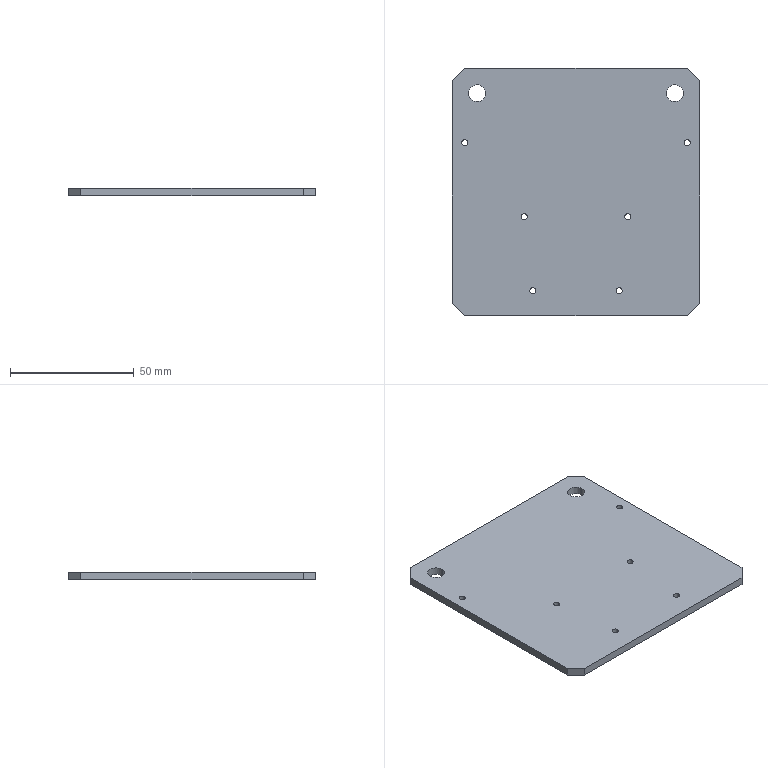Part | STEP file | J013-EBZ05-15-06-Part-1 | 1 solid | 26 faces | box 100 x 100 x 3.2 mm | volume 31513 mm3 | cylinder 16 | plane 10 | commonest cylinder face diameters 2.5 x12 6.8 x4
STEP:
#1=CARTESIAN_POINT('',(68.75,-15.,3.2));
#2=VERTEX_POINT('',#1);
#3=CARTESIAN_POINT('',(66.25,-15.,3.2));
#4=VERTEX_POINT('',#3);
#5=CARTESIAN_POINT('',(67.5,-15.,3.2));
#6=DIRECTION('',(0.,0.,-1.));
#7=DIRECTION('',(-1.,0.,0.));
#8=AXIS2_PLACEMENT_3D('',#5,#6,#7);
#9=CIRCLE('',#8,1.25);
#10=EDGE_CURVE('',#2,#4,#9,.T.);
#11=ORIENTED_EDGE('',*,*,#10,.F.);
#12=CARTESIAN_POINT('',(68.75,-15.,0.));
#13=VERTEX_POINT('',#12);
#14=CARTESIAN_POINT('',(68.75,-15.,3.2));
#15=DIRECTION('',(0.,0.,-1.));
#16=VECTOR('',#15,1000.);
#17=LINE('',#14,#16);
#18=EDGE_CURVE('',#2,#13,#17,.T.);
#19=ORIENTED_EDGE('',*,*,#18,.T.);
#20=CARTESIAN_POINT('',(66.25,-15.,0.));
#21=VERTEX_POINT('',#20);
#22=CARTESIAN_POINT('',(67.5,-15.,0.));
#23=DIRECTION('',(0.,0.,1.));
#24=DIRECTION('',(1.,0.,0.));
#25=AXIS2_PLACEMENT_3D('',#22,#23,#24);
#26=CIRCLE('',#25,1.25);
#27=EDGE_CURVE('',#21,#13,#26,.T.);
#28=ORIENTED_EDGE('',*,*,#27,.F.);
#29=CARTESIAN_POINT('',(66.25,-15.,3.2));
#30=DIRECTION('',(0.,0.,-1.));
#31=VECTOR('',#30,1000.);
#32=LINE('',#29,#31);
#33=EDGE_CURVE('',#4,#21,#32,.T.);
#34=ORIENTED_EDGE('',*,*,#33,.F.);
#35=EDGE_LOOP('',(#11,#19,#28,#34));
#36=FACE_OUTER_BOUND('',#35,.T.);
#37=CARTESIAN_POINT('',(67.5,-15.,3.2));
#38=DIRECTION('',(0.,0.,-1.));
#39=DIRECTION('',(-1.,0.,0.));
#40=AXIS2_PLACEMENT_3D('',#37,#38,#39);
#41=CYLINDRICAL_SURFACE('',#40,1.25);
#42=ADVANCED_FACE('',(#36),#41,.F.);
#43=CARTESIAN_POINT('',(33.75,-15.,3.2));
#44=VERTEX_POINT('',#43);
#45=CARTESIAN_POINT('',(31.25,-15.,3.2));
#46=VERTEX_POINT('',#45);
#47=CARTESIAN_POINT('',(32.5,-15.,3.2));
#48=DIRECTION('',(0.,0.,-1.));
#49=DIRECTION('',(-1.,0.,0.));
#50=AXIS2_PLACEMENT_3D('',#47,#48,#49);
#51=CIRCLE('',#50,1.25);
#52=EDGE_CURVE('',#44,#46,#51,.T.);
#53=ORIENTED_EDGE('',*,*,#52,.F.);
#54=CARTESIAN_POINT('',(33.75,-15.,0.));
#55=VERTEX_POINT('',#54);
#56=CARTESIAN_POINT('',(33.75,-15.,3.2));
#57=DIRECTION('',(0.,0.,-1.));
#58=VECTOR('',#57,1000.);
#59=LINE('',#56,#58);
#60=EDGE_CURVE('',#44,#55,#59,.T.);
#61=ORIENTED_EDGE('',*,*,#60,.T.);
#62=CARTESIAN_POINT('',(31.25,-15.,0.));
#63=VERTEX_POINT('',#62);
#64=CARTESIAN_POINT('',(32.5,-15.,0.));
#65=DIRECTION('',(0.,0.,1.));
#66=DIRECTION('',(1.,0.,0.));
#67=AXIS2_PLACEMENT_3D('',#64,#65,#66);
#68=CIRCLE('',#67,1.25);
#69=EDGE_CURVE('',#63,#55,#68,.T.);
#70=ORIENTED_EDGE('',*,*,#69,.F.);
#71=CARTESIAN_POINT('',(31.25,-15.,3.2));
#72=DIRECTION('',(0.,0.,-1.));
#73=VECTOR('',#72,1000.);
#74=LINE('',#71,#73);
#75=EDGE_CURVE('',#46,#63,#74,.T.);
#76=ORIENTED_EDGE('',*,*,#75,.F.);
#77=EDGE_LOOP('',(#53,#61,#70,#76));
#78=FACE_OUTER_BOUND('',#77,.T.);
#79=CARTESIAN_POINT('',(32.5,-15.,3.2));
#80=DIRECTION('',(0.,0.,-1.));
#81=DIRECTION('',(-1.,0.,0.));
#82=AXIS2_PLACEMENT_3D('',#79,#80,#81);
#83=CYLINDRICAL_SURFACE('',#82,1.25);
#84=ADVANCED_FACE('',(#78),#83,.F.);
#85=CARTESIAN_POINT('',(72.25,15.,3.2));
#86=VERTEX_POINT('',#85);
#87=CARTESIAN_POINT('',(69.75,15.,3.2));
#88=VERTEX_POINT('',#87);
#89=CARTESIAN_POINT('',(71.,15.,3.2));
#90=DIRECTION('',(0.,0.,-1.));
#91=DIRECTION('',(-1.,0.,0.));
#92=AXIS2_PLACEMENT_3D('',#89,#90,#91);
#93=CIRCLE('',#92,1.25);
#94=EDGE_CURVE('',#86,#88,#93,.T.);
#95=ORIENTED_EDGE('',*,*,#94,.F.);
#96=CARTESIAN_POINT('',(72.25,15.,0.));
#97=VERTEX_POINT('',#96);
#98=CARTESIAN_POINT('',(72.25,15.,3.2));
#99=DIRECTION('',(0.,0.,-1.));
#100=VECTOR('',#99,1000.);
#101=LINE('',#98,#100);
#102=EDGE_CURVE('',#86,#97,#101,.T.);
#103=ORIENTED_EDGE('',*,*,#102,.T.);
#104=CARTESIAN_POINT('',(69.75,15.,0.));
#105=VERTEX_POINT('',#104);
#106=CARTESIAN_POINT('',(71.,15.,0.));
#107=DIRECTION('',(0.,0.,1.));
#108=DIRECTION('',(1.,0.,0.));
#109=AXIS2_PLACEMENT_3D('',#106,#107,#108);
#110=CIRCLE('',#109,1.25);
#111=EDGE_CURVE('',#105,#97,#110,.T.);
#112=ORIENTED_EDGE('',*,*,#111,.F.);
#113=CARTESIAN_POINT('',(69.75,15.,3.2));
#114=DIRECTION('',(0.,0.,-1.));
#115=VECTOR('',#114,1000.);
#116=LINE('',#113,#115);
#117=EDGE_CURVE('',#88,#105,#116,.T.);
#118=ORIENTED_EDGE('',*,*,#117,.F.);
#119=EDGE_LOOP('',(#95,#103,#112,#118));
#120=FACE_OUTER_BOUND('',#119,.T.);
#121=CARTESIAN_POINT('',(71.,15.,3.2));
#122=DIRECTION('',(0.,0.,-1.));
#123=DIRECTION('',(-1.,0.,0.));
#124=AXIS2_PLACEMENT_3D('',#121,#122,#123);
#125=CYLINDRICAL_SURFACE('',#124,1.25);
#126=ADVANCED_FACE('',(#120),#125,.F.);
#127=CARTESIAN_POINT('',(30.25,15.,3.2));
#128=VERTEX_POINT('',#127);
#129=CARTESIAN_POINT('',(27.75,15.,3.2));
#130=VERTEX_POINT('',#129);
#131=CARTESIAN_POINT('',(29.,15.,3.2));
#132=DIRECTION('',(0.,0.,-1.));
#133=DIRECTION('',(-1.,0.,0.));
#134=AXIS2_PLACEMENT_3D('',#131,#132,#133);
#135=CIRCLE('',#134,1.25);
#136=EDGE_CURVE('',#128,#130,#135,.T.);
#137=ORIENTED_EDGE('',*,*,#136,.F.);
#138=CARTESIAN_POINT('',(30.25,15.,0.));
#139=VERTEX_POINT('',#138);
#140=CARTESIAN_POINT('',(30.25,15.,3.2));
#141=DIRECTION('',(0.,0.,-1.));
#142=VECTOR('',#141,1000.);
#143=LINE('',#140,#142);
#144=EDGE_CURVE('',#128,#139,#143,.T.);
#145=ORIENTED_EDGE('',*,*,#144,.T.);
#146=CARTESIAN_POINT('',(27.75,15.,0.));
#147=VERTEX_POINT('',#146);
#148=CARTESIAN_POINT('',(29.,15.,0.));
#149=DIRECTION('',(0.,0.,1.));
#150=DIRECTION('',(1.,0.,0.));
#151=AXIS2_PLACEMENT_3D('',#148,#149,#150);
#152=CIRCLE('',#151,1.25);
#153=EDGE_CURVE('',#147,#139,#152,.T.);
#154=ORIENTED_EDGE('',*,*,#153,.F.);
#155=CARTESIAN_POINT('',(27.75,15.,3.2));
#156=DIRECTION('',(0.,0.,-1.));
#157=VECTOR('',#156,1000.);
#158=LINE('',#155,#157);
#159=EDGE_CURVE('',#130,#147,#158,.T.);
#160=ORIENTED_EDGE('',*,*,#159,.F.);
#161=EDGE_LOOP('',(#137,#145,#154,#160));
#162=FACE_OUTER_BOUND('',#161,.T.);
#163=CARTESIAN_POINT('',(29.,15.,3.2));
#164=DIRECTION('',(0.,0.,-1.));
#165=DIRECTION('',(-1.,0.,0.));
#166=AXIS2_PLACEMENT_3D('',#163,#164,#165);
#167=CYLINDRICAL_SURFACE('',#166,1.25);
#168=ADVANCED_FACE('',(#162),#167,.F.);
#169=CARTESIAN_POINT('',(96.25,45.,3.2));
#170=VERTEX_POINT('',#169);
#171=CARTESIAN_POINT('',(93.75,45.,3.2));
#172=VERTEX_POINT('',#171);
#173=CARTESIAN_POINT('',(95.,45.,3.2));
#174=DIRECTION('',(0.,0.,-1.));
#175=DIRECTION('',(-1.,0.,0.));
#176=AXIS2_PLACEMENT_3D('',#173,#174,#175);
#177=CIRCLE('',#176,1.25);
#178=EDGE_CURVE('',#170,#172,#177,.T.);
#179=ORIENTED_EDGE('',*,*,#178,.F.);
#180=CARTESIAN_POINT('',(96.25,45.,0.));
#181=VERTEX_POINT('',#180);
#182=CARTESIAN_POINT('',(96.25,45.,3.2));
#183=DIRECTION('',(0.,0.,-1.));
#184=VECTOR('',#183,1000.);
#185=LINE('',#182,#184);
#186=EDGE_CURVE('',#170,#181,#185,.T.);
#187=ORIENTED_EDGE('',*,*,#186,.T.);
#188=CARTESIAN_POINT('',(93.75,45.,0.));
#189=VERTEX_POINT('',#188);
#190=CARTESIAN_POINT('',(95.,45.,0.));
#191=DIRECTION('',(0.,0.,1.));
#192=DIRECTION('',(1.,0.,0.));
#193=AXIS2_PLACEMENT_3D('',#190,#191,#192);
#194=CIRCLE('',#193,1.25);
#195=EDGE_CURVE('',#189,#181,#194,.T.);
#196=ORIENTED_EDGE('',*,*,#195,.F.);
#197=CARTESIAN_POINT('',(93.75,45.,3.2));
#198=DIRECTION('',(0.,0.,-1.));
#199=VECTOR('',#198,1000.);
#200=LINE('',#197,#199);
#201=EDGE_CURVE('',#172,#189,#200,.T.);
#202=ORIENTED_EDGE('',*,*,#201,.F.);
#203=EDGE_LOOP('',(#179,#187,#196,#202));
#204=FACE_OUTER_BOUND('',#203,.T.);
#205=CARTESIAN_POINT('',(95.,45.,3.2));
#206=DIRECTION('',(0.,0.,-1.));
#207=DIRECTION('',(-1.,0.,0.));
#208=AXIS2_PLACEMENT_3D('',#205,#206,#207);
#209=CYLINDRICAL_SURFACE('',#208,1.25);
#210=ADVANCED_FACE('',(#204),#209,.F.);
#211=CARTESIAN_POINT('',(6.25,45.,3.2));
#212=VERTEX_POINT('',#211);
#213=CARTESIAN_POINT('',(3.75,45.,3.2));
#214=VERTEX_POINT('',#213);
#215=CARTESIAN_POINT('',(5.,45.,3.2));
#216=DIRECTION('',(0.,0.,-1.));
#217=DIRECTION('',(-1.,0.,0.));
#218=AXIS2_PLACEMENT_3D('',#215,#216,#217);
#219=CIRCLE('',#218,1.25);
#220=EDGE_CURVE('',#212,#214,#219,.T.);
#221=ORIENTED_EDGE('',*,*,#220,.F.);
#222=CARTESIAN_POINT('',(6.25,45.,0.));
#223=VERTEX_POINT('',#222);
#224=CARTESIAN_POINT('',(6.25,45.,3.2));
#225=DIRECTION('',(0.,0.,-1.));
#226=VECTOR('',#225,1000.);
#227=LINE('',#224,#226);
#228=EDGE_CURVE('',#212,#223,#227,.T.);
#229=ORIENTED_EDGE('',*,*,#228,.T.);
#230=CARTESIAN_POINT('',(3.75,45.,0.));
#231=VERTEX_POINT('',#230);
#232=CARTESIAN_POINT('',(5.,45.,0.));
#233=DIRECTION('',(0.,0.,1.));
#234=DIRECTION('',(1.,0.,0.));
#235=AXIS2_PLACEMENT_3D('',#232,#233,#234);
#236=CIRCLE('',#235,1.25);
#237=EDGE_CURVE('',#231,#223,#236,.T.);
#238=ORIENTED_EDGE('',*,*,#237,.F.);
#239=CARTESIAN_POINT('',(3.75,45.,3.2));
#240=DIRECTION('',(0.,0.,-1.));
#241=VECTOR('',#240,1000.);
#242=LINE('',#239,#241);
#243=EDGE_CURVE('',#214,#231,#242,.T.);
#244=ORIENTED_EDGE('',*,*,#243,.F.);
#245=EDGE_LOOP('',(#221,#229,#238,#244));
#246=FACE_OUTER_BOUND('',#245,.T.);
#247=CARTESIAN_POINT('',(5.,45.,3.2));
#248=DIRECTION('',(0.,0.,-1.));
#249=DIRECTION('',(-1.,0.,0.));
#250=AXIS2_PLACEMENT_3D('',#247,#248,#249);
#251=CYLINDRICAL_SURFACE('',#250,1.25);
#252=ADVANCED_FACE('',(#246),#251,.F.);
#253=CARTESIAN_POINT('',(13.4,65.,3.2));
#254=VERTEX_POINT('',#253);
#255=CARTESIAN_POINT('',(6.6,65.,3.2));
#256=VERTEX_POINT('',#255);
#257=CARTESIAN_POINT('',(10.,65.,3.2));
#258=DIRECTION('',(0.,0.,-1.));
#259=DIRECTION('',(-1.,0.,0.));
#260=AXIS2_PLACEMENT_3D('',#257,#258,#259);
#261=CIRCLE('',#260,3.4);
#262=EDGE_CURVE('',#254,#256,#261,.T.);
#263=ORIENTED_EDGE('',*,*,#262,.F.);
#264=CARTESIAN_POINT('',(13.4,65.,0.));
#265=VERTEX_POINT('',#264);
#266=CARTESIAN_POINT('',(13.4,65.,3.2));
#267=DIRECTION('',(0.,0.,-1.));
#268=VECTOR('',#267,1000.);
#269=LINE('',#266,#268);
#270=EDGE_CURVE('',#254,#265,#269,.T.);
#271=ORIENTED_EDGE('',*,*,#270,.T.);
#272=CARTESIAN_POINT('',(6.6,65.,0.));
#273=VERTEX_POINT('',#272);
#274=CARTESIAN_POINT('',(10.,65.,0.));
#275=DIRECTION('',(0.,0.,1.));
#276=DIRECTION('',(1.,0.,0.));
#277=AXIS2_PLACEMENT_3D('',#274,#275,#276);
#278=CIRCLE('',#277,3.4);
#279=EDGE_CURVE('',#273,#265,#278,.T.);
#280=ORIENTED_EDGE('',*,*,#279,.F.);
#281=CARTESIAN_POINT('',(6.6,65.,3.2));
#282=DIRECTION('',(0.,0.,-1.));
#283=VECTOR('',#282,1000.);
#284=LINE('',#281,#283);
#285=EDGE_CURVE('',#256,#273,#284,.T.);
#286=ORIENTED_EDGE('',*,*,#285,.F.);
#287=EDGE_LOOP('',(#263,#271,#280,#286));
#288=FACE_OUTER_BOUND('',#287,.T.);
#289=CARTESIAN_POINT('',(10.,65.,3.2));
#290=DIRECTION('',(0.,0.,-1.));
#291=DIRECTION('',(-1.,0.,0.));
#292=AXIS2_PLACEMENT_3D('',#289,#290,#291);
#293=CYLINDRICAL_SURFACE('',#292,3.4);
#294=ADVANCED_FACE('',(#288),#293,.F.);
#295=CARTESIAN_POINT('',(93.4,65.,3.2));
#296=VERTEX_POINT('',#295);
#297=CARTESIAN_POINT('',(86.6,65.,3.2));
#298=VERTEX_POINT('',#297);
#299=CARTESIAN_POINT('',(90.,65.,3.2));
#300=DIRECTION('',(0.,0.,-1.));
#301=DIRECTION('',(-1.,0.,0.));
#302=AXIS2_PLACEMENT_3D('',#299,#300,#301);
#303=CIRCLE('',#302,3.4);
#304=EDGE_CURVE('',#296,#298,#303,.T.);
#305=ORIENTED_EDGE('',*,*,#304,.F.);
#306=CARTESIAN_POINT('',(93.4,65.,0.));
#307=VERTEX_POINT('',#306);
#308=CARTESIAN_POINT('',(93.4,65.,3.2));
#309=DIRECTION('',(0.,0.,-1.));
#310=VECTOR('',#309,1000.);
#311=LINE('',#308,#310);
#312=EDGE_CURVE('',#296,#307,#311,.T.);
#313=ORIENTED_EDGE('',*,*,#312,.T.);
#314=CARTESIAN_POINT('',(86.6,65.,0.));
#315=VERTEX_POINT('',#314);
#316=CARTESIAN_POINT('',(90.,65.,0.));
#317=DIRECTION('',(0.,0.,1.));
#318=DIRECTION('',(1.,0.,0.));
#319=AXIS2_PLACEMENT_3D('',#316,#317,#318);
#320=CIRCLE('',#319,3.4);
#321=EDGE_CURVE('',#315,#307,#320,.T.);
#322=ORIENTED_EDGE('',*,*,#321,.F.);
#323=CARTESIAN_POINT('',(86.6,65.,3.2));
#324=DIRECTION('',(0.,0.,-1.));
#325=VECTOR('',#324,1000.);
#326=LINE('',#323,#325);
#327=EDGE_CURVE('',#298,#315,#326,.T.);
#328=ORIENTED_EDGE('',*,*,#327,.F.);
#329=EDGE_LOOP('',(#305,#313,#322,#328));
#330=FACE_OUTER_BOUND('',#329,.T.);
#331=CARTESIAN_POINT('',(90.,65.,3.2));
#332=DIRECTION('',(0.,0.,-1.));
#333=DIRECTION('',(-1.,0.,0.));
#334=AXIS2_PLACEMENT_3D('',#331,#332,#333);
#335=CYLINDRICAL_SURFACE('',#334,3.4);
#336=ADVANCED_FACE('',(#330),#335,.F.);
#337=CARTESIAN_POINT('',(67.5,-15.,3.2));
#338=DIRECTION('',(0.,0.,-1.));
#339=DIRECTION('',(-1.,0.,0.));
#340=AXIS2_PLACEMENT_3D('',#337,#338,#339);
#341=CIRCLE('',#340,1.25);
#342=EDGE_CURVE('',#4,#2,#341,.T.);
#343=ORIENTED_EDGE('',*,*,#342,.T.);
#344=ORIENTED_EDGE('',*,*,#10,.T.);
#345=EDGE_LOOP('',(#343,#344));
#346=FACE_BOUND('',#345,.T.);
#347=CARTESIAN_POINT('',(32.5,-15.,3.2));
#348=DIRECTION('',(0.,0.,-1.));
#349=DIRECTION('',(-1.,0.,0.));
#350=AXIS2_PLACEMENT_3D('',#347,#348,#349);
#351=CIRCLE('',#350,1.25);
#352=EDGE_CURVE('',#46,#44,#351,.T.);
#353=ORIENTED_EDGE('',*,*,#352,.T.);
#354=ORIENTED_EDGE('',*,*,#52,.T.);
#355=EDGE_LOOP('',(#353,#354));
#356=FACE_BOUND('',#355,.T.);
#357=CARTESIAN_POINT('',(71.,15.,3.2));
#358=DIRECTION('',(0.,0.,-1.));
#359=DIRECTION('',(-1.,0.,0.));
#360=AXIS2_PLACEMENT_3D('',#357,#358,#359);
#361=CIRCLE('',#360,1.25);
#362=EDGE_CURVE('',#88,#86,#361,.T.);
#363=ORIENTED_EDGE('',*,*,#362,.T.);
#364=ORIENTED_EDGE('',*,*,#94,.T.);
#365=EDGE_LOOP('',(#363,#364));
#366=FACE_BOUND('',#365,.T.);
#367=CARTESIAN_POINT('',(29.,15.,3.2));
#368=DIRECTION('',(0.,0.,-1.));
#369=DIRECTION('',(-1.,0.,0.));
#370=AXIS2_PLACEMENT_3D('',#367,#368,#369);
#371=CIRCLE('',#370,1.25);
#372=EDGE_CURVE('',#130,#128,#371,.T.);
#373=ORIENTED_EDGE('',*,*,#372,.T.);
#374=ORIENTED_EDGE('',*,*,#136,.T.);
#375=EDGE_LOOP('',(#373,#374));
#376=FACE_BOUND('',#375,.T.);
#377=CARTESIAN_POINT('',(95.,45.,3.2));
#378=DIRECTION('',(0.,0.,-1.));
#379=DIRECTION('',(-1.,0.,0.));
#380=AXIS2_PLACEMENT_3D('',#377,#378,#379);
#381=CIRCLE('',#380,1.25);
#382=EDGE_CURVE('',#172,#170,#381,.T.);
#383=ORIENTED_EDGE('',*,*,#382,.T.);
#384=ORIENTED_EDGE('',*,*,#178,.T.);
#385=EDGE_LOOP('',(#383,#384));
#386=FACE_BOUND('',#385,.T.);
#387=CARTESIAN_POINT('',(5.,45.,3.2));
#388=DIRECTION('',(0.,0.,-1.));
#389=DIRECTION('',(-1.,0.,0.));
#390=AXIS2_PLACEMENT_3D('',#387,#388,#389);
#391=CIRCLE('',#390,1.25);
#392=EDGE_CURVE('',#214,#212,#391,.T.);
#393=ORIENTED_EDGE('',*,*,#392,.T.);
#394=ORIENTED_EDGE('',*,*,#220,.T.);
#395=EDGE_LOOP('',(#393,#394));
#396=FACE_BOUND('',#395,.T.);
#397=CARTESIAN_POINT('',(10.,65.,3.2));
#398=DIRECTION('',(0.,0.,-1.));
#399=DIRECTION('',(-1.,0.,0.));
#400=AXIS2_PLACEMENT_3D('',#397,#398,#399);
#401=CIRCLE('',#400,3.4);
#402=EDGE_CURVE('',#256,#254,#401,.T.);
#403=ORIENTED_EDGE('',*,*,#402,.T.);
#404=ORIENTED_EDGE('',*,*,#262,.T.);
#405=EDGE_LOOP('',(#403,#404));
#406=FACE_BOUND('',#405,.T.);
#407=CARTESIAN_POINT('',(90.,65.,3.2));
#408=DIRECTION('',(0.,0.,-1.));
#409=DIRECTION('',(-1.,0.,0.));
#410=AXIS2_PLACEMENT_3D('',#407,#408,#409);
#411=CIRCLE('',#410,3.4);
#412=EDGE_CURVE('',#298,#296,#411,.T.);
#413=ORIENTED_EDGE('',*,*,#412,.T.);
#414=ORIENTED_EDGE('',*,*,#304,.T.);
#415=EDGE_LOOP('',(#413,#414));
#416=FACE_BOUND('',#415,.T.);
#417=CARTESIAN_POINT('',(95.,-25.,3.2));
#418=VERTEX_POINT('',#417);
#419=CARTESIAN_POINT('',(5.,-25.,3.2));
#420=VERTEX_POINT('',#419);
#421=CARTESIAN_POINT('',(50.,-25.,3.2));
#422=DIRECTION('',(-1.,0.,0.));
#423=VECTOR('',#422,1000.);
#424=LINE('',#421,#423);
#425=EDGE_CURVE('',#418,#420,#424,.T.);
#426=ORIENTED_EDGE('',*,*,#425,.F.);
#427=CARTESIAN_POINT('',(100.,-20.,3.2));
#428=VERTEX_POINT('',#427);
#429=CARTESIAN_POINT('',(97.5,-22.5,3.2));
#430=DIRECTION('',(0.7071,0.7071,0.));
#431=VECTOR('',#430,1000.);
#432=LINE('',#429,#431);
#433=EDGE_CURVE('',#418,#428,#432,.T.);
#434=ORIENTED_EDGE('',*,*,#433,.T.);
#435=CARTESIAN_POINT('',(100.,70.,3.2));
#436=VERTEX_POINT('',#435);
#437=CARTESIAN_POINT('',(100.,25.,3.2));
#438=DIRECTION('',(0.,-1.,0.));
#439=VECTOR('',#438,1000.);
#440=LINE('',#437,#439);
#441=EDGE_CURVE('',#436,#428,#440,.T.);
#442=ORIENTED_EDGE('',*,*,#441,.F.);
#443=CARTESIAN_POINT('',(95.,75.,3.2));
#444=VERTEX_POINT('',#443);
#445=CARTESIAN_POINT('',(97.5,72.5,3.2));
#446=DIRECTION('',(-0.7071,0.7071,0.));
#447=VECTOR('',#446,1000.);
#448=LINE('',#445,#447);
#449=EDGE_CURVE('',#436,#444,#448,.T.);
#450=ORIENTED_EDGE('',*,*,#449,.T.);
#451=CARTESIAN_POINT('',(5.,75.,3.2));
#452=VERTEX_POINT('',#451);
#453=CARTESIAN_POINT('',(50.,75.,3.2));
#454=DIRECTION('',(1.,0.,0.));
#455=VECTOR('',#454,1000.);
#456=LINE('',#453,#455);
#457=EDGE_CURVE('',#452,#444,#456,.T.);
#458=ORIENTED_EDGE('',*,*,#457,.F.);
#459=CARTESIAN_POINT('',(0.,70.,3.2));
#460=VERTEX_POINT('',#459);
#461=CARTESIAN_POINT('',(2.5,72.5,3.2));
#462=DIRECTION('',(-0.7071,-0.7071,0.));
#463=VECTOR('',#462,1000.);
#464=LINE('',#461,#463);
#465=EDGE_CURVE('',#452,#460,#464,.T.);
#466=ORIENTED_EDGE('',*,*,#465,.T.);
#467=CARTESIAN_POINT('',(0.,-20.,3.2));
#468=VERTEX_POINT('',#467);
#469=CARTESIAN_POINT('',(0.,25.,3.2));
#470=DIRECTION('',(0.,1.,0.));
#471=VECTOR('',#470,1000.);
#472=LINE('',#469,#471);
#473=EDGE_CURVE('',#468,#460,#472,.T.);
#474=ORIENTED_EDGE('',*,*,#473,.F.);
#475=CARTESIAN_POINT('',(2.5,-22.5,3.2));
#476=DIRECTION('',(0.7071,-0.7071,0.));
#477=VECTOR('',#476,1000.);
#478=LINE('',#475,#477);
#479=EDGE_CURVE('',#468,#420,#478,.T.);
#480=ORIENTED_EDGE('',*,*,#479,.T.);
#481=EDGE_LOOP('',(#426,#434,#442,#450,#458,#466,#474,#480));
#482=FACE_OUTER_BOUND('',#481,.T.);
#483=CARTESIAN_POINT('',(50.,25.,3.2));
#484=DIRECTION('',(0.,0.,1.));
#485=DIRECTION('',(1.,0.,0.));
#486=AXIS2_PLACEMENT_3D('',#483,#484,#485);
#487=PLANE('',#486);
#488=ADVANCED_FACE('',(#346,#356,#366,#376,#386,#396,#406,#416,#482),#487,.T.);
#489=CARTESIAN_POINT('',(5.,-25.,0.));
#490=VERTEX_POINT('',#489);
#491=CARTESIAN_POINT('',(95.,-25.,0.));
#492=VERTEX_POINT('',#491);
#493=CARTESIAN_POINT('',(50.,-25.,0.));
#494=DIRECTION('',(1.,0.,0.));
#495=VECTOR('',#494,1000.);
#496=LINE('',#493,#495);
#497=EDGE_CURVE('',#490,#492,#496,.T.);
#498=ORIENTED_EDGE('',*,*,#497,.T.);
#499=CARTESIAN_POINT('',(95.,-25.,0.));
#500=DIRECTION('',(0.,0.,1.));
#501=VECTOR('',#500,1000.);
#502=LINE('',#499,#501);
#503=EDGE_CURVE('',#492,#418,#502,.T.);
#504=ORIENTED_EDGE('',*,*,#503,.T.);
#505=ORIENTED_EDGE('',*,*,#425,.T.);
#506=CARTESIAN_POINT('',(5.,-25.,0.));
#507=DIRECTION('',(0.,0.,-1.));
#508=VECTOR('',#507,1000.);
#509=LINE('',#506,#508);
#510=EDGE_CURVE('',#420,#490,#509,.T.);
#511=ORIENTED_EDGE('',*,*,#510,.T.);
#512=EDGE_LOOP('',(#498,#504,#505,#511));
#513=FACE_OUTER_BOUND('',#512,.T.);
#514=CARTESIAN_POINT('',(50.,-25.,0.));
#515=DIRECTION('',(0.,-1.,0.));
#516=DIRECTION('',(0.,0.,-1.));
#517=AXIS2_PLACEMENT_3D('',#514,#515,#516);
#518=PLANE('',#517);
#519=ADVANCED_FACE('',(#513),#518,.T.);
#520=CARTESIAN_POINT('',(0.,70.,0.));
#521=VERTEX_POINT('',#520);
#522=CARTESIAN_POINT('',(0.,-20.,0.));
#523=VERTEX_POINT('',#522);
#524=CARTESIAN_POINT('',(0.,25.,0.));
#525=DIRECTION('',(0.,-1.,0.));
#526=VECTOR('',#525,1000.);
#527=LINE('',#524,#526);
#528=EDGE_CURVE('',#521,#523,#527,.T.);
#529=ORIENTED_EDGE('',*,*,#528,.T.);
#530=CARTESIAN_POINT('',(0.,-20.,0.));
#531=DIRECTION('',(0.,0.,1.));
#532=VECTOR('',#531,1000.);
#533=LINE('',#530,#532);
#534=EDGE_CURVE('',#523,#468,#533,.T.);
#535=ORIENTED_EDGE('',*,*,#534,.T.);
#536=ORIENTED_EDGE('',*,*,#473,.T.);
#537=CARTESIAN_POINT('',(0.,70.,0.));
#538=DIRECTION('',(0.,0.,-1.));
#539=VECTOR('',#538,1000.);
#540=LINE('',#537,#539);
#541=EDGE_CURVE('',#460,#521,#540,.T.);
#542=ORIENTED_EDGE('',*,*,#541,.T.);
#543=EDGE_LOOP('',(#529,#535,#536,#542));
#544=FACE_OUTER_BOUND('',#543,.T.);
#545=CARTESIAN_POINT('',(0.,25.,0.));
#546=DIRECTION('',(-1.,0.,0.));
#547=DIRECTION('',(0.,0.,1.));
#548=AXIS2_PLACEMENT_3D('',#545,#546,#547);
#549=PLANE('',#548);
#550=ADVANCED_FACE('',(#544),#549,.T.);
#551=ORIENTED_EDGE('',*,*,#457,.T.);
#552=CARTESIAN_POINT('',(95.,75.,0.));
#553=VERTEX_POINT('',#552);
#554=CARTESIAN_POINT('',(95.,75.,0.));
#555=DIRECTION('',(0.,0.,-1.));
#556=VECTOR('',#555,1000.);
#557=LINE('',#554,#556);
#558=EDGE_CURVE('',#444,#553,#557,.T.);
#559=ORIENTED_EDGE('',*,*,#558,.T.);
#560=CARTESIAN_POINT('',(5.,75.,0.));
#561=VERTEX_POINT('',#560);
#562=CARTESIAN_POINT('',(50.,75.,0.));
#563=DIRECTION('',(-1.,0.,0.));
#564=VECTOR('',#563,1000.);
#565=LINE('',#562,#564);
#566=EDGE_CURVE('',#553,#561,#565,.T.);
#567=ORIENTED_EDGE('',*,*,#566,.T.);
#568=CARTESIAN_POINT('',(5.,75.,0.));
#569=DIRECTION('',(0.,0.,1.));
#570=VECTOR('',#569,1000.);
#571=LINE('',#568,#570);
#572=EDGE_CURVE('',#561,#452,#571,.T.);
#573=ORIENTED_EDGE('',*,*,#572,.T.);
#574=EDGE_LOOP('',(#551,#559,#567,#573));
#575=FACE_OUTER_BOUND('',#574,.T.);
#576=CARTESIAN_POINT('',(50.,75.,0.));
#577=DIRECTION('',(0.,1.,0.));
#578=DIRECTION('',(0.,0.,1.));
#579=AXIS2_PLACEMENT_3D('',#576,#577,#578);
#580=PLANE('',#579);
#581=ADVANCED_FACE('',(#575),#580,.T.);
#582=ORIENTED_EDGE('',*,*,#27,.T.);
#583=CARTESIAN_POINT('',(67.5,-15.,0.));
#584=DIRECTION('',(0.,0.,1.));
#585=DIRECTION('',(1.,0.,0.));
#586=AXIS2_PLACEMENT_3D('',#583,#584,#585);
#587=CIRCLE('',#586,1.25);
#588=EDGE_CURVE('',#13,#21,#587,.T.);
#589=ORIENTED_EDGE('',*,*,#588,.T.);
#590=EDGE_LOOP('',(#582,#589));
#591=FACE_BOUND('',#590,.T.);
#592=ORIENTED_EDGE('',*,*,#69,.T.);
#593=CARTESIAN_POINT('',(32.5,-15.,0.));
#594=DIRECTION('',(0.,0.,1.));
#595=DIRECTION('',(1.,0.,0.));
#596=AXIS2_PLACEMENT_3D('',#593,#594,#595);
#597=CIRCLE('',#596,1.25);
#598=EDGE_CURVE('',#55,#63,#597,.T.);
#599=ORIENTED_EDGE('',*,*,#598,.T.);
#600=EDGE_LOOP('',(#592,#599));
#601=FACE_BOUND('',#600,.T.);
#602=ORIENTED_EDGE('',*,*,#111,.T.);
#603=CARTESIAN_POINT('',(71.,15.,0.));
#604=DIRECTION('',(0.,0.,1.));
#605=DIRECTION('',(1.,0.,0.));
#606=AXIS2_PLACEMENT_3D('',#603,#604,#605);
#607=CIRCLE('',#606,1.25);
#608=EDGE_CURVE('',#97,#105,#607,.T.);
#609=ORIENTED_EDGE('',*,*,#608,.T.);
#610=EDGE_LOOP('',(#602,#609));
#611=FACE_BOUND('',#610,.T.);
#612=ORIENTED_EDGE('',*,*,#153,.T.);
#613=CARTESIAN_POINT('',(29.,15.,0.));
#614=DIRECTION('',(0.,0.,1.));
#615=DIRECTION('',(1.,0.,0.));
#616=AXIS2_PLACEMENT_3D('',#613,#614,#615);
#617=CIRCLE('',#616,1.25);
#618=EDGE_CURVE('',#139,#147,#617,.T.);
#619=ORIENTED_EDGE('',*,*,#618,.T.);
#620=EDGE_LOOP('',(#612,#619));
#621=FACE_BOUND('',#620,.T.);
#622=ORIENTED_EDGE('',*,*,#195,.T.);
#623=CARTESIAN_POINT('',(95.,45.,0.));
#624=DIRECTION('',(0.,0.,1.));
#625=DIRECTION('',(1.,0.,0.));
#626=AXIS2_PLACEMENT_3D('',#623,#624,#625);
#627=CIRCLE('',#626,1.25);
#628=EDGE_CURVE('',#181,#189,#627,.T.);
#629=ORIENTED_EDGE('',*,*,#628,.T.);
#630=EDGE_LOOP('',(#622,#629));
#631=FACE_BOUND('',#630,.T.);
#632=ORIENTED_EDGE('',*,*,#237,.T.);
#633=CARTESIAN_POINT('',(5.,45.,0.));
#634=DIRECTION('',(0.,0.,1.));
#635=DIRECTION('',(1.,0.,0.));
#636=AXIS2_PLACEMENT_3D('',#633,#634,#635);
#637=CIRCLE('',#636,1.25);
#638=EDGE_CURVE('',#223,#231,#637,.T.);
#639=ORIENTED_EDGE('',*,*,#638,.T.);
#640=EDGE_LOOP('',(#632,#639));
#641=FACE_BOUND('',#640,.T.);
#642=ORIENTED_EDGE('',*,*,#279,.T.);
#643=CARTESIAN_POINT('',(10.,65.,0.));
#644=DIRECTION('',(0.,0.,1.));
#645=DIRECTION('',(1.,0.,0.));
#646=AXIS2_PLACEMENT_3D('',#643,#644,#645);
#647=CIRCLE('',#646,3.4);
#648=EDGE_CURVE('',#265,#273,#647,.T.);
#649=ORIENTED_EDGE('',*,*,#648,.T.);
#650=EDGE_LOOP('',(#642,#649));
#651=FACE_BOUND('',#650,.T.);
#652=ORIENTED_EDGE('',*,*,#321,.T.);
#653=CARTESIAN_POINT('',(90.,65.,0.));
#654=DIRECTION('',(0.,0.,1.));
#655=DIRECTION('',(1.,0.,0.));
#656=AXIS2_PLACEMENT_3D('',#653,#654,#655);
#657=CIRCLE('',#656,3.4);
#658=EDGE_CURVE('',#307,#315,#657,.T.);
#659=ORIENTED_EDGE('',*,*,#658,.T.);
#660=EDGE_LOOP('',(#652,#659));
#661=FACE_BOUND('',#660,.T.);
#662=CARTESIAN_POINT('',(100.,-20.,0.));
#663=VERTEX_POINT('',#662);
#664=CARTESIAN_POINT('',(100.,70.,0.));
#665=VERTEX_POINT('',#664);
#666=CARTESIAN_POINT('',(100.,25.,0.));
#667=DIRECTION('',(0.,1.,0.));
#668=VECTOR('',#667,1000.);
#669=LINE('',#666,#668);
#670=EDGE_CURVE('',#663,#665,#669,.T.);
#671=ORIENTED_EDGE('',*,*,#670,.F.);
#672=CARTESIAN_POINT('',(97.5,-22.5,0.));
#673=DIRECTION('',(-0.7071,-0.7071,0.));
#674=VECTOR('',#673,1000.);
#675=LINE('',#672,#674);
#676=EDGE_CURVE('',#663,#492,#675,.T.);
#677=ORIENTED_EDGE('',*,*,#676,.T.);
#678=ORIENTED_EDGE('',*,*,#497,.F.);
#679=CARTESIAN_POINT('',(2.5,-22.5,0.));
#680=DIRECTION('',(-0.7071,0.7071,0.));
#681=VECTOR('',#680,1000.);
#682=LINE('',#679,#681);
#683=EDGE_CURVE('',#490,#523,#682,.T.);
#684=ORIENTED_EDGE('',*,*,#683,.T.);
#685=ORIENTED_EDGE('',*,*,#528,.F.);
#686=CARTESIAN_POINT('',(2.5,72.5,0.));
#687=DIRECTION('',(0.7071,0.7071,0.));
#688=VECTOR('',#687,1000.);
#689=LINE('',#686,#688);
#690=EDGE_CURVE('',#521,#561,#689,.T.);
#691=ORIENTED_EDGE('',*,*,#690,.T.);
#692=ORIENTED_EDGE('',*,*,#566,.F.);
#693=CARTESIAN_POINT('',(97.5,72.5,0.));
#694=DIRECTION('',(0.7071,-0.7071,0.));
#695=VECTOR('',#694,1000.);
#696=LINE('',#693,#695);
#697=EDGE_CURVE('',#553,#665,#696,.T.);
#698=ORIENTED_EDGE('',*,*,#697,.T.);
#699=EDGE_LOOP('',(#671,#677,#678,#684,#685,#691,#692,#698));
#700=FACE_OUTER_BOUND('',#699,.T.);
#701=CARTESIAN_POINT('',(50.,25.,0.));
#702=DIRECTION('',(0.,0.,-1.));
#703=DIRECTION('',(-1.,0.,0.));
#704=AXIS2_PLACEMENT_3D('',#701,#702,#703);
#705=PLANE('',#704);
#706=ADVANCED_FACE('',(#591,#601,#611,#621,#631,#641,#651,#661,#700),#705,.T.);
#707=ORIENTED_EDGE('',*,*,#441,.T.);
#708=CARTESIAN_POINT('',(100.,-20.,0.));
#709=DIRECTION('',(0.,0.,-1.));
#710=VECTOR('',#709,1000.);
#711=LINE('',#708,#710);
#712=EDGE_CURVE('',#428,#663,#711,.T.);
#713=ORIENTED_EDGE('',*,*,#712,.T.);
#714=ORIENTED_EDGE('',*,*,#670,.T.);
#715=CARTESIAN_POINT('',(100.,70.,0.));
#716=DIRECTION('',(0.,0.,1.));
#717=VECTOR('',#716,1000.);
#718=LINE('',#715,#717);
#719=EDGE_CURVE('',#665,#436,#718,.T.);
#720=ORIENTED_EDGE('',*,*,#719,.T.);
#721=EDGE_LOOP('',(#707,#713,#714,#720));
#722=FACE_OUTER_BOUND('',#721,.T.);
#723=CARTESIAN_POINT('',(100.,25.,0.));
#724=DIRECTION('',(1.,0.,0.));
#725=DIRECTION('',(0.,0.,-1.));
#726=AXIS2_PLACEMENT_3D('',#723,#724,#725);
#727=PLANE('',#726);
#728=ADVANCED_FACE('',(#722),#727,.T.);
#729=ORIENTED_EDGE('',*,*,#312,.F.);
#730=ORIENTED_EDGE('',*,*,#412,.F.);
#731=ORIENTED_EDGE('',*,*,#327,.T.);
#732=ORIENTED_EDGE('',*,*,#658,.F.);
#733=EDGE_LOOP('',(#729,#730,#731,#732));
#734=FACE_OUTER_BOUND('',#733,.T.);
#735=CARTESIAN_POINT('',(90.,65.,3.2));
#736=DIRECTION('',(0.,0.,-1.));
#737=DIRECTION('',(-1.,0.,0.));
#738=AXIS2_PLACEMENT_3D('',#735,#736,#737);
#739=CYLINDRICAL_SURFACE('',#738,3.4);
#740=ADVANCED_FACE('',(#734),#739,.F.);
#741=ORIENTED_EDGE('',*,*,#270,.F.);
#742=ORIENTED_EDGE('',*,*,#402,.F.);
#743=ORIENTED_EDGE('',*,*,#285,.T.);
#744=ORIENTED_EDGE('',*,*,#648,.F.);
#745=EDGE_LOOP('',(#741,#742,#743,#744));
#746=FACE_OUTER_BOUND('',#745,.T.);
#747=CARTESIAN_POINT('',(10.,65.,3.2));
#748=DIRECTION('',(0.,0.,-1.));
#749=DIRECTION('',(-1.,0.,0.));
#750=AXIS2_PLACEMENT_3D('',#747,#748,#749);
#751=CYLINDRICAL_SURFACE('',#750,3.4);
#752=ADVANCED_FACE('',(#746),#751,.F.);
#753=ORIENTED_EDGE('',*,*,#690,.F.);
#754=ORIENTED_EDGE('',*,*,#541,.F.);
#755=ORIENTED_EDGE('',*,*,#465,.F.);
#756=ORIENTED_EDGE('',*,*,#572,.F.);
#757=EDGE_LOOP('',(#753,#754,#755,#756));
#758=FACE_OUTER_BOUND('',#757,.T.);
#759=CARTESIAN_POINT('',(5.,75.,0.));
#760=DIRECTION('',(0.7071,-0.7071,0.));
#761=DIRECTION('',(0.,0.,1.));
#762=AXIS2_PLACEMENT_3D('',#759,#760,#761);
#763=PLANE('',#762);
#764=ADVANCED_FACE('',(#758),#763,.F.);
#765=ORIENTED_EDGE('',*,*,#683,.F.);
#766=ORIENTED_EDGE('',*,*,#510,.F.);
#767=ORIENTED_EDGE('',*,*,#479,.F.);
#768=ORIENTED_EDGE('',*,*,#534,.F.);
#769=EDGE_LOOP('',(#765,#766,#767,#768));
#770=FACE_OUTER_BOUND('',#769,.T.);
#771=CARTESIAN_POINT('',(0.,-20.,0.));
#772=DIRECTION('',(0.7071,0.7071,0.));
#773=DIRECTION('',(0.,0.,1.));
#774=AXIS2_PLACEMENT_3D('',#771,#772,#773);
#775=PLANE('',#774);
#776=ADVANCED_FACE('',(#770),#775,.F.);
#777=ORIENTED_EDGE('',*,*,#697,.F.);
#778=ORIENTED_EDGE('',*,*,#558,.F.);
#779=ORIENTED_EDGE('',*,*,#449,.F.);
#780=ORIENTED_EDGE('',*,*,#719,.F.);
#781=EDGE_LOOP('',(#777,#778,#779,#780));
#782=FACE_OUTER_BOUND('',#781,.T.);
#783=CARTESIAN_POINT('',(100.,70.,0.));
#784=DIRECTION('',(-0.7071,-0.7071,0.));
#785=DIRECTION('',(0.,0.,1.));
#786=AXIS2_PLACEMENT_3D('',#783,#784,#785);
#787=PLANE('',#786);
#788=ADVANCED_FACE('',(#782),#787,.F.);
#789=ORIENTED_EDGE('',*,*,#676,.F.);
#790=ORIENTED_EDGE('',*,*,#712,.F.);
#791=ORIENTED_EDGE('',*,*,#433,.F.);
#792=ORIENTED_EDGE('',*,*,#503,.F.);
#793=EDGE_LOOP('',(#789,#790,#791,#792));
#794=FACE_OUTER_BOUND('',#793,.T.);
#795=CARTESIAN_POINT('',(95.,-25.,0.));
#796=DIRECTION('',(-0.7071,0.7071,0.));
#797=DIRECTION('',(0.,0.,1.));
#798=AXIS2_PLACEMENT_3D('',#795,#796,#797);
#799=PLANE('',#798);
#800=ADVANCED_FACE('',(#794),#799,.F.);
#801=ORIENTED_EDGE('',*,*,#228,.F.);
#802=ORIENTED_EDGE('',*,*,#392,.F.);
#803=ORIENTED_EDGE('',*,*,#243,.T.);
#804=ORIENTED_EDGE('',*,*,#638,.F.);
#805=EDGE_LOOP('',(#801,#802,#803,#804));
#806=FACE_OUTER_BOUND('',#805,.T.);
#807=CARTESIAN_POINT('',(5.,45.,3.2));
#808=DIRECTION('',(0.,0.,-1.));
#809=DIRECTION('',(-1.,0.,0.));
#810=AXIS2_PLACEMENT_3D('',#807,#808,#809);
#811=CYLINDRICAL_SURFACE('',#810,1.25);
#812=ADVANCED_FACE('',(#806),#811,.F.);
#813=ORIENTED_EDGE('',*,*,#186,.F.);
#814=ORIENTED_EDGE('',*,*,#382,.F.);
#815=ORIENTED_EDGE('',*,*,#201,.T.);
#816=ORIENTED_EDGE('',*,*,#628,.F.);
#817=EDGE_LOOP('',(#813,#814,#815,#816));
#818=FACE_OUTER_BOUND('',#817,.T.);
#819=CARTESIAN_POINT('',(95.,45.,3.2));
#820=DIRECTION('',(0.,0.,-1.));
#821=DIRECTION('',(-1.,0.,0.));
#822=AXIS2_PLACEMENT_3D('',#819,#820,#821);
#823=CYLINDRICAL_SURFACE('',#822,1.25);
#824=ADVANCED_FACE('',(#818),#823,.F.);
#825=ORIENTED_EDGE('',*,*,#144,.F.);
#826=ORIENTED_EDGE('',*,*,#372,.F.);
#827=ORIENTED_EDGE('',*,*,#159,.T.);
#828=ORIENTED_EDGE('',*,*,#618,.F.);
#829=EDGE_LOOP('',(#825,#826,#827,#828));
#830=FACE_OUTER_BOUND('',#829,.T.);
#831=CARTESIAN_POINT('',(29.,15.,3.2));
#832=DIRECTION('',(0.,0.,-1.));
#833=DIRECTION('',(-1.,0.,0.));
#834=AXIS2_PLACEMENT_3D('',#831,#832,#833);
#835=CYLINDRICAL_SURFACE('',#834,1.25);
#836=ADVANCED_FACE('',(#830),#835,.F.);
#837=ORIENTED_EDGE('',*,*,#102,.F.);
#838=ORIENTED_EDGE('',*,*,#362,.F.);
#839=ORIENTED_EDGE('',*,*,#117,.T.);
#840=ORIENTED_EDGE('',*,*,#608,.F.);
#841=EDGE_LOOP('',(#837,#838,#839,#840));
#842=FACE_OUTER_BOUND('',#841,.T.);
#843=CARTESIAN_POINT('',(71.,15.,3.2));
#844=DIRECTION('',(0.,0.,-1.));
#845=DIRECTION('',(-1.,0.,0.));
#846=AXIS2_PLACEMENT_3D('',#843,#844,#845);
#847=CYLINDRICAL_SURFACE('',#846,1.25);
#848=ADVANCED_FACE('',(#842),#847,.F.);
#849=ORIENTED_EDGE('',*,*,#60,.F.);
#850=ORIENTED_EDGE('',*,*,#352,.F.);
#851=ORIENTED_EDGE('',*,*,#75,.T.);
#852=ORIENTED_EDGE('',*,*,#598,.F.);
#853=EDGE_LOOP('',(#849,#850,#851,#852));
#854=FACE_OUTER_BOUND('',#853,.T.);
#855=CARTESIAN_POINT('',(32.5,-15.,3.2));
#856=DIRECTION('',(0.,0.,-1.));
#857=DIRECTION('',(-1.,0.,0.));
#858=AXIS2_PLACEMENT_3D('',#855,#856,#857);
#859=CYLINDRICAL_SURFACE('',#858,1.25);
#860=ADVANCED_FACE('',(#854),#859,.F.);
#861=ORIENTED_EDGE('',*,*,#18,.F.);
#862=ORIENTED_EDGE('',*,*,#342,.F.);
#863=ORIENTED_EDGE('',*,*,#33,.T.);
#864=ORIENTED_EDGE('',*,*,#588,.F.);
#865=EDGE_LOOP('',(#861,#862,#863,#864));
#866=FACE_OUTER_BOUND('',#865,.T.);
#867=CARTESIAN_POINT('',(67.5,-15.,3.2));
#868=DIRECTION('',(0.,0.,-1.));
#869=DIRECTION('',(-1.,0.,0.));
#870=AXIS2_PLACEMENT_3D('',#867,#868,#869);
#871=CYLINDRICAL_SURFACE('',#870,1.25);
#872=ADVANCED_FACE('',(#866),#871,.F.);
#873=CLOSED_SHELL('',(#42,#84,#126,#168,#210,#252,#294,#336,#488,#519,#550,#581,#706,#728,#740,#752,#764,#776,#788,#800,#812,#824,#836,#848,#860,#872));
#874=MANIFOLD_SOLID_BREP('',#873);
#875=CARTESIAN_POINT('',(0.,0.,0.));
#876=DIRECTION('',(0.,0.,1.));
#877=DIRECTION('',(1.,0.,0.));
#878=AXIS2_PLACEMENT_3D('',#875,#876,#877);
#879=(LENGTH_UNIT()NAMED_UNIT(*)SI_UNIT(.MILLI.,.METRE.));
#880=UNCERTAINTY_MEASURE_WITH_UNIT(LENGTH_MEASURE(0.00001),#879,'','');
#881=(NAMED_UNIT(*)PLANE_ANGLE_UNIT()SI_UNIT($,.RADIAN.));
#882=(NAMED_UNIT(*)SI_UNIT($,.STERADIAN.)SOLID_ANGLE_UNIT());
#883=(GEOMETRIC_REPRESENTATION_CONTEXT(3)GLOBAL_UNCERTAINTY_ASSIGNED_CONTEXT((#880))GLOBAL_UNIT_ASSIGNED_CONTEXT((#879,#881,#882))REPRESENTATION_CONTEXT('',''));
#884=ADVANCED_BREP_SHAPE_REPRESENTATION('',(#874,#878),#883);